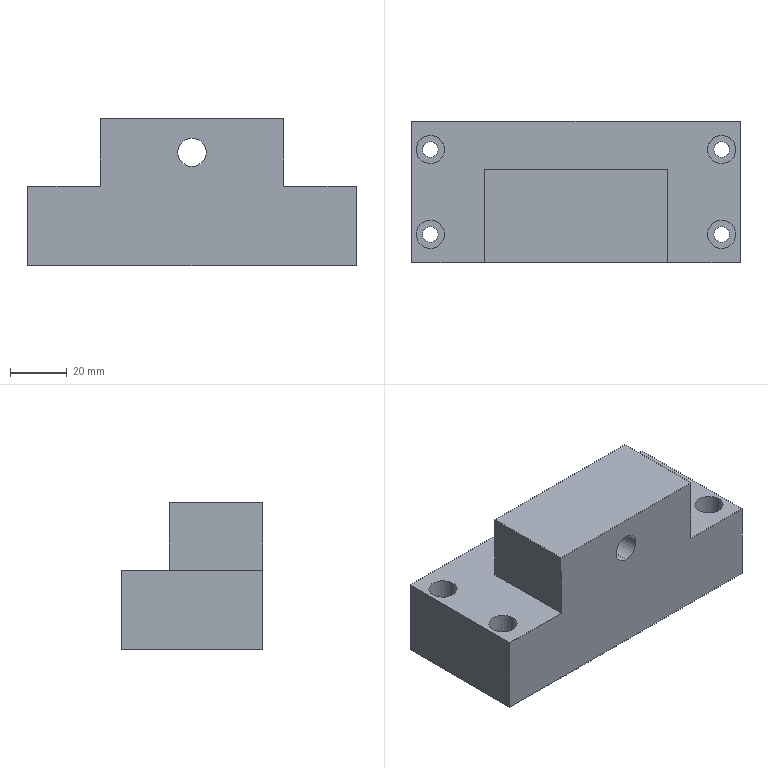Part | 1 solid | 36 faces | box 116 x 50 x 52 mm | volume 203244 mm3 | cylinder 20 | plane 14 | cone 2 | commonest cylinder face diameters 10 x10 5.5 x8 8.5 x2
STEP:
#1=CARTESIAN_POINT('',(46.5,-15.,10.));
#2=VERTEX_POINT('',#1);
#3=CARTESIAN_POINT('',(56.5,-15.,10.));
#4=VERTEX_POINT('',#3);
#5=CARTESIAN_POINT('',(51.5,-15.,10.));
#6=DIRECTION('',(0.,0.,1.));
#7=DIRECTION('',(1.,0.,0.));
#8=AXIS2_PLACEMENT_3D('',#5,#6,#7);
#9=CIRCLE('',#8,5.);
#10=EDGE_CURVE('',#2,#4,#9,.T.);
#11=ORIENTED_EDGE('',*,*,#10,.F.);
#12=CARTESIAN_POINT('',(46.5,-15.,28.));
#13=VERTEX_POINT('',#12);
#14=CARTESIAN_POINT('',(46.5,-15.,28.));
#15=DIRECTION('',(0.,0.,1.));
#16=VECTOR('',#15,1000.);
#17=LINE('',#14,#16);
#18=EDGE_CURVE('',#2,#13,#17,.T.);
#19=ORIENTED_EDGE('',*,*,#18,.T.);
#20=CARTESIAN_POINT('',(56.5,-15.,28.));
#21=VERTEX_POINT('',#20);
#22=CARTESIAN_POINT('',(51.5,-15.,28.));
#23=DIRECTION('',(0.,0.,1.));
#24=DIRECTION('',(1.,0.,0.));
#25=AXIS2_PLACEMENT_3D('',#22,#23,#24);
#26=CIRCLE('',#25,5.);
#27=EDGE_CURVE('',#13,#21,#26,.T.);
#28=ORIENTED_EDGE('',*,*,#27,.T.);
#29=CARTESIAN_POINT('',(56.5,-15.,28.));
#30=DIRECTION('',(0.,0.,1.));
#31=VECTOR('',#30,1000.);
#32=LINE('',#29,#31);
#33=EDGE_CURVE('',#4,#21,#32,.T.);
#34=ORIENTED_EDGE('',*,*,#33,.F.);
#35=EDGE_LOOP('',(#11,#19,#28,#34));
#36=FACE_OUTER_BOUND('',#35,.T.);
#37=CARTESIAN_POINT('',(51.5,-15.,28.));
#38=DIRECTION('',(0.,0.,1.));
#39=DIRECTION('',(1.,0.,0.));
#40=AXIS2_PLACEMENT_3D('',#37,#38,#39);
#41=CYLINDRICAL_SURFACE('',#40,5.);
#42=ADVANCED_FACE('',(#36),#41,.F.);
#43=CARTESIAN_POINT('',(48.75,-15.,0.));
#44=VERTEX_POINT('',#43);
#45=CARTESIAN_POINT('',(54.25,-15.,0.));
#46=VERTEX_POINT('',#45);
#47=CARTESIAN_POINT('',(51.5,-15.,0.));
#48=DIRECTION('',(0.,0.,1.));
#49=DIRECTION('',(1.,0.,0.));
#50=AXIS2_PLACEMENT_3D('',#47,#48,#49);
#51=CIRCLE('',#50,2.75);
#52=EDGE_CURVE('',#44,#46,#51,.T.);
#53=ORIENTED_EDGE('',*,*,#52,.F.);
#54=CARTESIAN_POINT('',(48.75,-15.,10.));
#55=VERTEX_POINT('',#54);
#56=CARTESIAN_POINT('',(48.75,-15.,28.));
#57=DIRECTION('',(0.,0.,1.));
#58=VECTOR('',#57,1000.);
#59=LINE('',#56,#58);
#60=EDGE_CURVE('',#44,#55,#59,.T.);
#61=ORIENTED_EDGE('',*,*,#60,.T.);
#62=CARTESIAN_POINT('',(54.25,-15.,10.));
#63=VERTEX_POINT('',#62);
#64=CARTESIAN_POINT('',(51.5,-15.,10.));
#65=DIRECTION('',(0.,0.,1.));
#66=DIRECTION('',(1.,0.,0.));
#67=AXIS2_PLACEMENT_3D('',#64,#65,#66);
#68=CIRCLE('',#67,2.75);
#69=EDGE_CURVE('',#55,#63,#68,.T.);
#70=ORIENTED_EDGE('',*,*,#69,.T.);
#71=CARTESIAN_POINT('',(54.25,-15.,28.));
#72=DIRECTION('',(0.,0.,1.));
#73=VECTOR('',#72,1000.);
#74=LINE('',#71,#73);
#75=EDGE_CURVE('',#46,#63,#74,.T.);
#76=ORIENTED_EDGE('',*,*,#75,.F.);
#77=EDGE_LOOP('',(#53,#61,#70,#76));
#78=FACE_OUTER_BOUND('',#77,.T.);
#79=CARTESIAN_POINT('',(51.5,-15.,28.));
#80=DIRECTION('',(0.,0.,1.));
#81=DIRECTION('',(1.,0.,0.));
#82=AXIS2_PLACEMENT_3D('',#79,#80,#81);
#83=CYLINDRICAL_SURFACE('',#82,2.75);
#84=ADVANCED_FACE('',(#78),#83,.F.);
#85=CARTESIAN_POINT('',(46.5,15.,10.));
#86=VERTEX_POINT('',#85);
#87=CARTESIAN_POINT('',(56.5,15.,10.));
#88=VERTEX_POINT('',#87);
#89=CARTESIAN_POINT('',(51.5,15.,10.));
#90=DIRECTION('',(0.,0.,1.));
#91=DIRECTION('',(1.,0.,0.));
#92=AXIS2_PLACEMENT_3D('',#89,#90,#91);
#93=CIRCLE('',#92,5.);
#94=EDGE_CURVE('',#86,#88,#93,.T.);
#95=ORIENTED_EDGE('',*,*,#94,.F.);
#96=CARTESIAN_POINT('',(46.5,15.,28.));
#97=VERTEX_POINT('',#96);
#98=CARTESIAN_POINT('',(46.5,15.,28.));
#99=DIRECTION('',(0.,0.,1.));
#100=VECTOR('',#99,1000.);
#101=LINE('',#98,#100);
#102=EDGE_CURVE('',#86,#97,#101,.T.);
#103=ORIENTED_EDGE('',*,*,#102,.T.);
#104=CARTESIAN_POINT('',(56.5,15.,28.));
#105=VERTEX_POINT('',#104);
#106=CARTESIAN_POINT('',(51.5,15.,28.));
#107=DIRECTION('',(0.,0.,1.));
#108=DIRECTION('',(1.,0.,0.));
#109=AXIS2_PLACEMENT_3D('',#106,#107,#108);
#110=CIRCLE('',#109,5.);
#111=EDGE_CURVE('',#97,#105,#110,.T.);
#112=ORIENTED_EDGE('',*,*,#111,.T.);
#113=CARTESIAN_POINT('',(56.5,15.,28.));
#114=DIRECTION('',(0.,0.,1.));
#115=VECTOR('',#114,1000.);
#116=LINE('',#113,#115);
#117=EDGE_CURVE('',#88,#105,#116,.T.);
#118=ORIENTED_EDGE('',*,*,#117,.F.);
#119=EDGE_LOOP('',(#95,#103,#112,#118));
#120=FACE_OUTER_BOUND('',#119,.T.);
#121=CARTESIAN_POINT('',(51.5,15.,28.));
#122=DIRECTION('',(0.,0.,1.));
#123=DIRECTION('',(1.,0.,0.));
#124=AXIS2_PLACEMENT_3D('',#121,#122,#123);
#125=CYLINDRICAL_SURFACE('',#124,5.);
#126=ADVANCED_FACE('',(#120),#125,.F.);
#127=CARTESIAN_POINT('',(48.75,15.,0.));
#128=VERTEX_POINT('',#127);
#129=CARTESIAN_POINT('',(54.25,15.,0.));
#130=VERTEX_POINT('',#129);
#131=CARTESIAN_POINT('',(51.5,15.,0.));
#132=DIRECTION('',(0.,0.,1.));
#133=DIRECTION('',(1.,0.,0.));
#134=AXIS2_PLACEMENT_3D('',#131,#132,#133);
#135=CIRCLE('',#134,2.75);
#136=EDGE_CURVE('',#128,#130,#135,.T.);
#137=ORIENTED_EDGE('',*,*,#136,.F.);
#138=CARTESIAN_POINT('',(48.75,15.,10.));
#139=VERTEX_POINT('',#138);
#140=CARTESIAN_POINT('',(48.75,15.,28.));
#141=DIRECTION('',(0.,0.,1.));
#142=VECTOR('',#141,1000.);
#143=LINE('',#140,#142);
#144=EDGE_CURVE('',#128,#139,#143,.T.);
#145=ORIENTED_EDGE('',*,*,#144,.T.);
#146=CARTESIAN_POINT('',(54.25,15.,10.));
#147=VERTEX_POINT('',#146);
#148=CARTESIAN_POINT('',(51.5,15.,10.));
#149=DIRECTION('',(0.,0.,1.));
#150=DIRECTION('',(1.,0.,0.));
#151=AXIS2_PLACEMENT_3D('',#148,#149,#150);
#152=CIRCLE('',#151,2.75);
#153=EDGE_CURVE('',#139,#147,#152,.T.);
#154=ORIENTED_EDGE('',*,*,#153,.T.);
#155=CARTESIAN_POINT('',(54.25,15.,28.));
#156=DIRECTION('',(0.,0.,1.));
#157=VECTOR('',#156,1000.);
#158=LINE('',#155,#157);
#159=EDGE_CURVE('',#130,#147,#158,.T.);
#160=ORIENTED_EDGE('',*,*,#159,.F.);
#161=EDGE_LOOP('',(#137,#145,#154,#160));
#162=FACE_OUTER_BOUND('',#161,.T.);
#163=CARTESIAN_POINT('',(51.5,15.,28.));
#164=DIRECTION('',(0.,0.,1.));
#165=DIRECTION('',(1.,0.,0.));
#166=AXIS2_PLACEMENT_3D('',#163,#164,#165);
#167=CYLINDRICAL_SURFACE('',#166,2.75);
#168=ADVANCED_FACE('',(#162),#167,.F.);
#169=CARTESIAN_POINT('',(-56.5,-15.,10.));
#170=VERTEX_POINT('',#169);
#171=CARTESIAN_POINT('',(-46.5,-15.,10.));
#172=VERTEX_POINT('',#171);
#173=CARTESIAN_POINT('',(-51.5,-15.,10.));
#174=DIRECTION('',(0.,0.,1.));
#175=DIRECTION('',(1.,0.,0.));
#176=AXIS2_PLACEMENT_3D('',#173,#174,#175);
#177=CIRCLE('',#176,5.);
#178=EDGE_CURVE('',#170,#172,#177,.T.);
#179=ORIENTED_EDGE('',*,*,#178,.F.);
#180=CARTESIAN_POINT('',(-56.5,-15.,28.));
#181=VERTEX_POINT('',#180);
#182=CARTESIAN_POINT('',(-56.5,-15.,28.));
#183=DIRECTION('',(0.,0.,1.));
#184=VECTOR('',#183,1000.);
#185=LINE('',#182,#184);
#186=EDGE_CURVE('',#170,#181,#185,.T.);
#187=ORIENTED_EDGE('',*,*,#186,.T.);
#188=CARTESIAN_POINT('',(-46.5,-15.,28.));
#189=VERTEX_POINT('',#188);
#190=CARTESIAN_POINT('',(-51.5,-15.,28.));
#191=DIRECTION('',(0.,0.,1.));
#192=DIRECTION('',(1.,0.,0.));
#193=AXIS2_PLACEMENT_3D('',#190,#191,#192);
#194=CIRCLE('',#193,5.);
#195=EDGE_CURVE('',#181,#189,#194,.T.);
#196=ORIENTED_EDGE('',*,*,#195,.T.);
#197=CARTESIAN_POINT('',(-46.5,-15.,28.));
#198=DIRECTION('',(0.,0.,1.));
#199=VECTOR('',#198,1000.);
#200=LINE('',#197,#199);
#201=EDGE_CURVE('',#172,#189,#200,.T.);
#202=ORIENTED_EDGE('',*,*,#201,.F.);
#203=EDGE_LOOP('',(#179,#187,#196,#202));
#204=FACE_OUTER_BOUND('',#203,.T.);
#205=CARTESIAN_POINT('',(-51.5,-15.,28.));
#206=DIRECTION('',(0.,0.,1.));
#207=DIRECTION('',(1.,0.,0.));
#208=AXIS2_PLACEMENT_3D('',#205,#206,#207);
#209=CYLINDRICAL_SURFACE('',#208,5.);
#210=ADVANCED_FACE('',(#204),#209,.F.);
#211=CARTESIAN_POINT('',(-54.25,-15.,0.));
#212=VERTEX_POINT('',#211);
#213=CARTESIAN_POINT('',(-48.75,-15.,0.));
#214=VERTEX_POINT('',#213);
#215=CARTESIAN_POINT('',(-51.5,-15.,0.));
#216=DIRECTION('',(0.,0.,1.));
#217=DIRECTION('',(1.,0.,0.));
#218=AXIS2_PLACEMENT_3D('',#215,#216,#217);
#219=CIRCLE('',#218,2.75);
#220=EDGE_CURVE('',#212,#214,#219,.T.);
#221=ORIENTED_EDGE('',*,*,#220,.F.);
#222=CARTESIAN_POINT('',(-54.25,-15.,10.));
#223=VERTEX_POINT('',#222);
#224=CARTESIAN_POINT('',(-54.25,-15.,28.));
#225=DIRECTION('',(0.,0.,1.));
#226=VECTOR('',#225,1000.);
#227=LINE('',#224,#226);
#228=EDGE_CURVE('',#212,#223,#227,.T.);
#229=ORIENTED_EDGE('',*,*,#228,.T.);
#230=CARTESIAN_POINT('',(-48.75,-15.,10.));
#231=VERTEX_POINT('',#230);
#232=CARTESIAN_POINT('',(-51.5,-15.,10.));
#233=DIRECTION('',(0.,0.,1.));
#234=DIRECTION('',(1.,0.,0.));
#235=AXIS2_PLACEMENT_3D('',#232,#233,#234);
#236=CIRCLE('',#235,2.75);
#237=EDGE_CURVE('',#223,#231,#236,.T.);
#238=ORIENTED_EDGE('',*,*,#237,.T.);
#239=CARTESIAN_POINT('',(-48.75,-15.,28.));
#240=DIRECTION('',(0.,0.,1.));
#241=VECTOR('',#240,1000.);
#242=LINE('',#239,#241);
#243=EDGE_CURVE('',#214,#231,#242,.T.);
#244=ORIENTED_EDGE('',*,*,#243,.F.);
#245=EDGE_LOOP('',(#221,#229,#238,#244));
#246=FACE_OUTER_BOUND('',#245,.T.);
#247=CARTESIAN_POINT('',(-51.5,-15.,28.));
#248=DIRECTION('',(0.,0.,1.));
#249=DIRECTION('',(1.,0.,0.));
#250=AXIS2_PLACEMENT_3D('',#247,#248,#249);
#251=CYLINDRICAL_SURFACE('',#250,2.75);
#252=ADVANCED_FACE('',(#246),#251,.F.);
#253=CARTESIAN_POINT('',(-56.5,15.,10.));
#254=VERTEX_POINT('',#253);
#255=CARTESIAN_POINT('',(-46.5,15.,10.));
#256=VERTEX_POINT('',#255);
#257=CARTESIAN_POINT('',(-51.5,15.,10.));
#258=DIRECTION('',(0.,0.,1.));
#259=DIRECTION('',(1.,0.,0.));
#260=AXIS2_PLACEMENT_3D('',#257,#258,#259);
#261=CIRCLE('',#260,5.);
#262=EDGE_CURVE('',#254,#256,#261,.T.);
#263=ORIENTED_EDGE('',*,*,#262,.F.);
#264=CARTESIAN_POINT('',(-56.5,15.,28.));
#265=VERTEX_POINT('',#264);
#266=CARTESIAN_POINT('',(-56.5,15.,28.));
#267=DIRECTION('',(0.,0.,1.));
#268=VECTOR('',#267,1000.);
#269=LINE('',#266,#268);
#270=EDGE_CURVE('',#254,#265,#269,.T.);
#271=ORIENTED_EDGE('',*,*,#270,.T.);
#272=CARTESIAN_POINT('',(-46.5,15.,28.));
#273=VERTEX_POINT('',#272);
#274=CARTESIAN_POINT('',(-51.5,15.,28.));
#275=DIRECTION('',(0.,0.,1.));
#276=DIRECTION('',(1.,0.,0.));
#277=AXIS2_PLACEMENT_3D('',#274,#275,#276);
#278=CIRCLE('',#277,5.);
#279=EDGE_CURVE('',#265,#273,#278,.T.);
#280=ORIENTED_EDGE('',*,*,#279,.T.);
#281=CARTESIAN_POINT('',(-46.5,15.,28.));
#282=DIRECTION('',(0.,0.,1.));
#283=VECTOR('',#282,1000.);
#284=LINE('',#281,#283);
#285=EDGE_CURVE('',#256,#273,#284,.T.);
#286=ORIENTED_EDGE('',*,*,#285,.F.);
#287=EDGE_LOOP('',(#263,#271,#280,#286));
#288=FACE_OUTER_BOUND('',#287,.T.);
#289=CARTESIAN_POINT('',(-51.5,15.,28.));
#290=DIRECTION('',(0.,0.,1.));
#291=DIRECTION('',(1.,0.,0.));
#292=AXIS2_PLACEMENT_3D('',#289,#290,#291);
#293=CYLINDRICAL_SURFACE('',#292,5.);
#294=ADVANCED_FACE('',(#288),#293,.F.);
#295=CARTESIAN_POINT('',(-54.25,15.,0.));
#296=VERTEX_POINT('',#295);
#297=CARTESIAN_POINT('',(-48.75,15.,0.));
#298=VERTEX_POINT('',#297);
#299=CARTESIAN_POINT('',(-51.5,15.,0.));
#300=DIRECTION('',(0.,0.,1.));
#301=DIRECTION('',(1.,0.,0.));
#302=AXIS2_PLACEMENT_3D('',#299,#300,#301);
#303=CIRCLE('',#302,2.75);
#304=EDGE_CURVE('',#296,#298,#303,.T.);
#305=ORIENTED_EDGE('',*,*,#304,.F.);
#306=CARTESIAN_POINT('',(-54.25,15.,10.));
#307=VERTEX_POINT('',#306);
#308=CARTESIAN_POINT('',(-54.25,15.,28.));
#309=DIRECTION('',(0.,0.,1.));
#310=VECTOR('',#309,1000.);
#311=LINE('',#308,#310);
#312=EDGE_CURVE('',#296,#307,#311,.T.);
#313=ORIENTED_EDGE('',*,*,#312,.T.);
#314=CARTESIAN_POINT('',(-48.75,15.,10.));
#315=VERTEX_POINT('',#314);
#316=CARTESIAN_POINT('',(-51.5,15.,10.));
#317=DIRECTION('',(0.,0.,1.));
#318=DIRECTION('',(1.,0.,0.));
#319=AXIS2_PLACEMENT_3D('',#316,#317,#318);
#320=CIRCLE('',#319,2.75);
#321=EDGE_CURVE('',#307,#315,#320,.T.);
#322=ORIENTED_EDGE('',*,*,#321,.T.);
#323=CARTESIAN_POINT('',(-48.75,15.,28.));
#324=DIRECTION('',(0.,0.,1.));
#325=VECTOR('',#324,1000.);
#326=LINE('',#323,#325);
#327=EDGE_CURVE('',#298,#315,#326,.T.);
#328=ORIENTED_EDGE('',*,*,#327,.F.);
#329=EDGE_LOOP('',(#305,#313,#322,#328));
#330=FACE_OUTER_BOUND('',#329,.T.);
#331=CARTESIAN_POINT('',(-51.5,15.,28.));
#332=DIRECTION('',(0.,0.,1.));
#333=DIRECTION('',(1.,0.,0.));
#334=AXIS2_PLACEMENT_3D('',#331,#332,#333);
#335=CYLINDRICAL_SURFACE('',#334,2.75);
#336=ADVANCED_FACE('',(#330),#335,.F.);
#337=CARTESIAN_POINT('',(0.,0.5,5.75));
#338=VERTEX_POINT('',#337);
#339=CARTESIAN_POINT('',(0.,0.5,14.25));
#340=VERTEX_POINT('',#339);
#341=CARTESIAN_POINT('',(0.,0.5,10.));
#342=DIRECTION('',(0.,1.,0.));
#343=DIRECTION('',(0.,0.,1.));
#344=AXIS2_PLACEMENT_3D('',#341,#342,#343);
#345=CIRCLE('',#344,4.25);
#346=EDGE_CURVE('',#338,#340,#345,.T.);
#347=ORIENTED_EDGE('',*,*,#346,.F.);
#348=CARTESIAN_POINT('',(0.,25.,5.75));
#349=VERTEX_POINT('',#348);
#350=CARTESIAN_POINT('',(0.,25.,5.75));
#351=DIRECTION('',(0.,1.,0.));
#352=VECTOR('',#351,1000.);
#353=LINE('',#350,#352);
#354=EDGE_CURVE('',#338,#349,#353,.T.);
#355=ORIENTED_EDGE('',*,*,#354,.T.);
#356=CARTESIAN_POINT('',(0.,25.,14.25));
#357=VERTEX_POINT('',#356);
#358=CARTESIAN_POINT('',(0.,25.,10.));
#359=DIRECTION('',(0.,1.,0.));
#360=DIRECTION('',(0.,0.,1.));
#361=AXIS2_PLACEMENT_3D('',#358,#359,#360);
#362=CIRCLE('',#361,4.25);
#363=EDGE_CURVE('',#349,#357,#362,.T.);
#364=ORIENTED_EDGE('',*,*,#363,.T.);
#365=CARTESIAN_POINT('',(0.,25.,14.25));
#366=DIRECTION('',(0.,1.,0.));
#367=VECTOR('',#366,1000.);
#368=LINE('',#365,#367);
#369=EDGE_CURVE('',#340,#357,#368,.T.);
#370=ORIENTED_EDGE('',*,*,#369,.F.);
#371=EDGE_LOOP('',(#347,#355,#364,#370));
#372=FACE_OUTER_BOUND('',#371,.T.);
#373=CARTESIAN_POINT('',(0.,25.,10.));
#374=DIRECTION('',(0.,1.,0.));
#375=DIRECTION('',(0.,0.,1.));
#376=AXIS2_PLACEMENT_3D('',#373,#374,#375);
#377=CYLINDRICAL_SURFACE('',#376,4.25);
#378=ADVANCED_FACE('',(#372),#377,.F.);
#379=CARTESIAN_POINT('',(0.,-2.054,10.));
#380=VERTEX_POINT('',#379);
#381=CARTESIAN_POINT('',(0.,0.5,14.25));
#382=DIRECTION('',(0.,0.515,0.8572));
#383=VECTOR('',#382,1000.);
#384=LINE('',#381,#383);
#385=EDGE_CURVE('',#380,#340,#384,.T.);
#386=ORIENTED_EDGE('',*,*,#385,.F.);
#387=CARTESIAN_POINT('',(0.,0.5,5.75));
#388=DIRECTION('',(0.,0.515,-0.8572));
#389=VECTOR('',#388,1000.);
#390=LINE('',#387,#389);
#391=EDGE_CURVE('',#380,#338,#390,.T.);
#392=ORIENTED_EDGE('',*,*,#391,.T.);
#393=ORIENTED_EDGE('',*,*,#346,.T.);
#394=EDGE_LOOP('',(#386,#392,#393));
#395=FACE_OUTER_BOUND('',#394,.T.);
#396=CARTESIAN_POINT('',(0.,0.5,10.));
#397=DIRECTION('',(0.,1.,0.));
#398=DIRECTION('',(0.,0.,1.));
#399=AXIS2_PLACEMENT_3D('',#396,#397,#398);
#400=CONICAL_SURFACE('',#399,4.25,1.03);
#401=ADVANCED_FACE('',(#395),#400,.F.);
#402=CARTESIAN_POINT('',(0.,-25.,35.));
#403=VERTEX_POINT('',#402);
#404=CARTESIAN_POINT('',(0.,-25.,45.));
#405=VERTEX_POINT('',#404);
#406=CARTESIAN_POINT('',(0.,-25.,40.));
#407=DIRECTION('',(0.,1.,0.));
#408=DIRECTION('',(0.,0.,1.));
#409=AXIS2_PLACEMENT_3D('',#406,#407,#408);
#410=CIRCLE('',#409,5.);
#411=EDGE_CURVE('',#403,#405,#410,.T.);
#412=ORIENTED_EDGE('',*,*,#411,.F.);
#413=CARTESIAN_POINT('',(0.,8.,35.));
#414=VERTEX_POINT('',#413);
#415=CARTESIAN_POINT('',(0.,8.,35.));
#416=DIRECTION('',(0.,1.,0.));
#417=VECTOR('',#416,1000.);
#418=LINE('',#415,#417);
#419=EDGE_CURVE('',#403,#414,#418,.T.);
#420=ORIENTED_EDGE('',*,*,#419,.T.);
#421=CARTESIAN_POINT('',(0.,8.,45.));
#422=VERTEX_POINT('',#421);
#423=CARTESIAN_POINT('',(0.,8.,40.));
#424=DIRECTION('',(0.,1.,0.));
#425=DIRECTION('',(0.,0.,1.));
#426=AXIS2_PLACEMENT_3D('',#423,#424,#425);
#427=CIRCLE('',#426,5.);
#428=EDGE_CURVE('',#414,#422,#427,.T.);
#429=ORIENTED_EDGE('',*,*,#428,.T.);
#430=CARTESIAN_POINT('',(0.,8.,45.));
#431=DIRECTION('',(0.,1.,0.));
#432=VECTOR('',#431,1000.);
#433=LINE('',#430,#432);
#434=EDGE_CURVE('',#405,#422,#433,.T.);
#435=ORIENTED_EDGE('',*,*,#434,.F.);
#436=EDGE_LOOP('',(#412,#420,#429,#435));
#437=FACE_OUTER_BOUND('',#436,.T.);
#438=CARTESIAN_POINT('',(0.,8.,40.));
#439=DIRECTION('',(0.,1.,0.));
#440=DIRECTION('',(0.,0.,1.));
#441=AXIS2_PLACEMENT_3D('',#438,#439,#440);
#442=CYLINDRICAL_SURFACE('',#441,5.);
#443=ADVANCED_FACE('',(#437),#442,.F.);
#444=CARTESIAN_POINT('',(51.5,-15.,28.));
#445=DIRECTION('',(0.,0.,1.));
#446=DIRECTION('',(1.,0.,0.));
#447=AXIS2_PLACEMENT_3D('',#444,#445,#446);
#448=CIRCLE('',#447,5.);
#449=EDGE_CURVE('',#21,#13,#448,.T.);
#450=ORIENTED_EDGE('',*,*,#449,.F.);
#451=ORIENTED_EDGE('',*,*,#27,.F.);
#452=EDGE_LOOP('',(#450,#451));
#453=FACE_BOUND('',#452,.T.);
#454=CARTESIAN_POINT('',(51.5,15.,28.));
#455=DIRECTION('',(0.,0.,1.));
#456=DIRECTION('',(1.,0.,0.));
#457=AXIS2_PLACEMENT_3D('',#454,#455,#456);
#458=CIRCLE('',#457,5.);
#459=EDGE_CURVE('',#105,#97,#458,.T.);
#460=ORIENTED_EDGE('',*,*,#459,.F.);
#461=ORIENTED_EDGE('',*,*,#111,.F.);
#462=EDGE_LOOP('',(#460,#461));
#463=FACE_BOUND('',#462,.T.);
#464=CARTESIAN_POINT('',(-51.5,-15.,28.));
#465=DIRECTION('',(0.,0.,1.));
#466=DIRECTION('',(1.,0.,0.));
#467=AXIS2_PLACEMENT_3D('',#464,#465,#466);
#468=CIRCLE('',#467,5.);
#469=EDGE_CURVE('',#189,#181,#468,.T.);
#470=ORIENTED_EDGE('',*,*,#469,.F.);
#471=ORIENTED_EDGE('',*,*,#195,.F.);
#472=EDGE_LOOP('',(#470,#471));
#473=FACE_BOUND('',#472,.T.);
#474=CARTESIAN_POINT('',(-51.5,15.,28.));
#475=DIRECTION('',(0.,0.,1.));
#476=DIRECTION('',(1.,0.,0.));
#477=AXIS2_PLACEMENT_3D('',#474,#475,#476);
#478=CIRCLE('',#477,5.);
#479=EDGE_CURVE('',#273,#265,#478,.T.);
#480=ORIENTED_EDGE('',*,*,#479,.F.);
#481=ORIENTED_EDGE('',*,*,#279,.F.);
#482=EDGE_LOOP('',(#480,#481));
#483=FACE_BOUND('',#482,.T.);
#484=CARTESIAN_POINT('',(-32.5,8.,28.));
#485=VERTEX_POINT('',#484);
#486=CARTESIAN_POINT('',(-32.5,-25.,28.));
#487=VERTEX_POINT('',#486);
#488=CARTESIAN_POINT('',(-32.5,-25.,28.));
#489=DIRECTION('',(0.,-1.,0.));
#490=VECTOR('',#489,1000.);
#491=LINE('',#488,#490);
#492=EDGE_CURVE('',#485,#487,#491,.T.);
#493=ORIENTED_EDGE('',*,*,#492,.F.);
#494=CARTESIAN_POINT('',(32.5,8.,28.));
#495=VERTEX_POINT('',#494);
#496=CARTESIAN_POINT('',(-32.5,8.,28.));
#497=DIRECTION('',(-1.,0.,0.));
#498=VECTOR('',#497,1000.);
#499=LINE('',#496,#498);
#500=EDGE_CURVE('',#495,#485,#499,.T.);
#501=ORIENTED_EDGE('',*,*,#500,.F.);
#502=CARTESIAN_POINT('',(32.5,-25.,28.));
#503=VERTEX_POINT('',#502);
#504=CARTESIAN_POINT('',(32.5,8.,28.));
#505=DIRECTION('',(0.,1.,0.));
#506=VECTOR('',#505,1000.);
#507=LINE('',#504,#506);
#508=EDGE_CURVE('',#503,#495,#507,.T.);
#509=ORIENTED_EDGE('',*,*,#508,.F.);
#510=CARTESIAN_POINT('',(58.,-25.,28.));
#511=VERTEX_POINT('',#510);
#512=CARTESIAN_POINT('',(58.,-25.,28.));
#513=DIRECTION('',(-1.,0.,0.));
#514=VECTOR('',#513,1000.);
#515=LINE('',#512,#514);
#516=EDGE_CURVE('',#511,#503,#515,.T.);
#517=ORIENTED_EDGE('',*,*,#516,.F.);
#518=CARTESIAN_POINT('',(58.,25.,28.));
#519=VERTEX_POINT('',#518);
#520=CARTESIAN_POINT('',(58.,25.,28.));
#521=DIRECTION('',(0.,-1.,0.));
#522=VECTOR('',#521,1000.);
#523=LINE('',#520,#522);
#524=EDGE_CURVE('',#519,#511,#523,.T.);
#525=ORIENTED_EDGE('',*,*,#524,.F.);
#526=CARTESIAN_POINT('',(-58.,25.,28.));
#527=VERTEX_POINT('',#526);
#528=CARTESIAN_POINT('',(-58.,25.,28.));
#529=DIRECTION('',(1.,0.,0.));
#530=VECTOR('',#529,1000.);
#531=LINE('',#528,#530);
#532=EDGE_CURVE('',#527,#519,#531,.T.);
#533=ORIENTED_EDGE('',*,*,#532,.F.);
#534=CARTESIAN_POINT('',(-58.,-25.,28.));
#535=VERTEX_POINT('',#534);
#536=CARTESIAN_POINT('',(-58.,-25.,28.));
#537=DIRECTION('',(0.,1.,0.));
#538=VECTOR('',#537,1000.);
#539=LINE('',#536,#538);
#540=EDGE_CURVE('',#535,#527,#539,.T.);
#541=ORIENTED_EDGE('',*,*,#540,.F.);
#542=CARTESIAN_POINT('',(58.,-25.,28.));
#543=DIRECTION('',(-1.,0.,0.));
#544=VECTOR('',#543,1000.);
#545=LINE('',#542,#544);
#546=EDGE_CURVE('',#487,#535,#545,.T.);
#547=ORIENTED_EDGE('',*,*,#546,.F.);
#548=EDGE_LOOP('',(#493,#501,#509,#517,#525,#533,#541,#547));
#549=FACE_OUTER_BOUND('',#548,.T.);
#550=CARTESIAN_POINT('',(0.,0.,28.));
#551=DIRECTION('',(0.,0.,-1.));
#552=DIRECTION('',(-1.,0.,0.));
#553=AXIS2_PLACEMENT_3D('',#550,#551,#552);
#554=PLANE('',#553);
#555=ADVANCED_FACE('',(#453,#463,#473,#483,#549),#554,.F.);
#556=CARTESIAN_POINT('',(0.,25.,10.));
#557=DIRECTION('',(0.,1.,0.));
#558=DIRECTION('',(0.,0.,1.));
#559=AXIS2_PLACEMENT_3D('',#556,#557,#558);
#560=CIRCLE('',#559,4.25);
#561=EDGE_CURVE('',#357,#349,#560,.T.);
#562=ORIENTED_EDGE('',*,*,#561,.F.);
#563=ORIENTED_EDGE('',*,*,#363,.F.);
#564=EDGE_LOOP('',(#562,#563));
#565=FACE_BOUND('',#564,.T.);
#566=CARTESIAN_POINT('',(-58.,25.,0.));
#567=VERTEX_POINT('',#566);
#568=CARTESIAN_POINT('',(58.,25.,0.));
#569=VERTEX_POINT('',#568);
#570=CARTESIAN_POINT('',(-58.,25.,0.));
#571=DIRECTION('',(1.,0.,0.));
#572=VECTOR('',#571,1000.);
#573=LINE('',#570,#572);
#574=EDGE_CURVE('',#567,#569,#573,.T.);
#575=ORIENTED_EDGE('',*,*,#574,.F.);
#576=CARTESIAN_POINT('',(-58.,25.,28.));
#577=DIRECTION('',(0.,0.,-1.));
#578=VECTOR('',#577,1000.);
#579=LINE('',#576,#578);
#580=EDGE_CURVE('',#527,#567,#579,.T.);
#581=ORIENTED_EDGE('',*,*,#580,.F.);
#582=ORIENTED_EDGE('',*,*,#532,.T.);
#583=CARTESIAN_POINT('',(58.,25.,28.));
#584=DIRECTION('',(0.,0.,-1.));
#585=VECTOR('',#584,1000.);
#586=LINE('',#583,#585);
#587=EDGE_CURVE('',#519,#569,#586,.T.);
#588=ORIENTED_EDGE('',*,*,#587,.T.);
#589=EDGE_LOOP('',(#575,#581,#582,#588));
#590=FACE_OUTER_BOUND('',#589,.T.);
#591=CARTESIAN_POINT('',(-58.,25.,28.));
#592=DIRECTION('',(0.,1.,0.));
#593=DIRECTION('',(0.,0.,1.));
#594=AXIS2_PLACEMENT_3D('',#591,#592,#593);
#595=PLANE('',#594);
#596=ADVANCED_FACE('',(#565,#590),#595,.T.);
#597=CARTESIAN_POINT('',(-58.,-25.,0.));
#598=VERTEX_POINT('',#597);
#599=CARTESIAN_POINT('',(-58.,-25.,0.));
#600=DIRECTION('',(0.,1.,0.));
#601=VECTOR('',#600,1000.);
#602=LINE('',#599,#601);
#603=EDGE_CURVE('',#598,#567,#602,.T.);
#604=ORIENTED_EDGE('',*,*,#603,.F.);
#605=CARTESIAN_POINT('',(-58.,-25.,28.));
#606=DIRECTION('',(0.,0.,-1.));
#607=VECTOR('',#606,1000.);
#608=LINE('',#605,#607);
#609=EDGE_CURVE('',#535,#598,#608,.T.);
#610=ORIENTED_EDGE('',*,*,#609,.F.);
#611=ORIENTED_EDGE('',*,*,#540,.T.);
#612=ORIENTED_EDGE('',*,*,#580,.T.);
#613=EDGE_LOOP('',(#604,#610,#611,#612));
#614=FACE_OUTER_BOUND('',#613,.T.);
#615=CARTESIAN_POINT('',(-58.,-25.,28.));
#616=DIRECTION('',(-1.,0.,0.));
#617=DIRECTION('',(0.,0.,1.));
#618=AXIS2_PLACEMENT_3D('',#615,#616,#617);
#619=PLANE('',#618);
#620=ADVANCED_FACE('',(#614),#619,.T.);
#621=CARTESIAN_POINT('',(0.,-25.,40.));
#622=DIRECTION('',(0.,1.,0.));
#623=DIRECTION('',(0.,0.,1.));
#624=AXIS2_PLACEMENT_3D('',#621,#622,#623);
#625=CIRCLE('',#624,5.);
#626=EDGE_CURVE('',#405,#403,#625,.T.);
#627=ORIENTED_EDGE('',*,*,#626,.T.);
#628=ORIENTED_EDGE('',*,*,#411,.T.);
#629=EDGE_LOOP('',(#627,#628));
#630=FACE_BOUND('',#629,.T.);
#631=CARTESIAN_POINT('',(58.,-25.,0.));
#632=VERTEX_POINT('',#631);
#633=CARTESIAN_POINT('',(58.,-25.,0.));
#634=DIRECTION('',(-1.,0.,0.));
#635=VECTOR('',#634,1000.);
#636=LINE('',#633,#635);
#637=EDGE_CURVE('',#632,#598,#636,.T.);
#638=ORIENTED_EDGE('',*,*,#637,.F.);
#639=CARTESIAN_POINT('',(58.,-25.,28.));
#640=DIRECTION('',(0.,0.,-1.));
#641=VECTOR('',#640,1000.);
#642=LINE('',#639,#641);
#643=EDGE_CURVE('',#511,#632,#642,.T.);
#644=ORIENTED_EDGE('',*,*,#643,.F.);
#645=ORIENTED_EDGE('',*,*,#516,.T.);
#646=CARTESIAN_POINT('',(32.5,-25.,52.));
#647=VERTEX_POINT('',#646);
#648=CARTESIAN_POINT('',(32.5,-25.,52.));
#649=DIRECTION('',(0.,0.,-1.));
#650=VECTOR('',#649,1000.);
#651=LINE('',#648,#650);
#652=EDGE_CURVE('',#647,#503,#651,.T.);
#653=ORIENTED_EDGE('',*,*,#652,.F.);
#654=CARTESIAN_POINT('',(-32.5,-25.,52.));
#655=VERTEX_POINT('',#654);
#656=CARTESIAN_POINT('',(32.5,-25.,52.));
#657=DIRECTION('',(1.,0.,0.));
#658=VECTOR('',#657,1000.);
#659=LINE('',#656,#658);
#660=EDGE_CURVE('',#655,#647,#659,.T.);
#661=ORIENTED_EDGE('',*,*,#660,.F.);
#662=CARTESIAN_POINT('',(-32.5,-25.,52.));
#663=DIRECTION('',(0.,0.,-1.));
#664=VECTOR('',#663,1000.);
#665=LINE('',#662,#664);
#666=EDGE_CURVE('',#655,#487,#665,.T.);
#667=ORIENTED_EDGE('',*,*,#666,.T.);
#668=ORIENTED_EDGE('',*,*,#546,.T.);
#669=ORIENTED_EDGE('',*,*,#609,.T.);
#670=EDGE_LOOP('',(#638,#644,#645,#653,#661,#667,#668,#669));
#671=FACE_OUTER_BOUND('',#670,.T.);
#672=CARTESIAN_POINT('',(58.,-25.,28.));
#673=DIRECTION('',(0.,-1.,0.));
#674=DIRECTION('',(0.,0.,-1.));
#675=AXIS2_PLACEMENT_3D('',#672,#673,#674);
#676=PLANE('',#675);
#677=ADVANCED_FACE('',(#630,#671),#676,.T.);
#678=CARTESIAN_POINT('',(58.,25.,0.));
#679=DIRECTION('',(0.,-1.,0.));
#680=VECTOR('',#679,1000.);
#681=LINE('',#678,#680);
#682=EDGE_CURVE('',#569,#632,#681,.T.);
#683=ORIENTED_EDGE('',*,*,#682,.F.);
#684=ORIENTED_EDGE('',*,*,#587,.F.);
#685=ORIENTED_EDGE('',*,*,#524,.T.);
#686=ORIENTED_EDGE('',*,*,#643,.T.);
#687=EDGE_LOOP('',(#683,#684,#685,#686));
#688=FACE_OUTER_BOUND('',#687,.T.);
#689=CARTESIAN_POINT('',(58.,25.,28.));
#690=DIRECTION('',(1.,0.,0.));
#691=DIRECTION('',(0.,0.,-1.));
#692=AXIS2_PLACEMENT_3D('',#689,#690,#691);
#693=PLANE('',#692);
#694=ADVANCED_FACE('',(#688),#693,.T.);
#695=CARTESIAN_POINT('',(51.5,-15.,0.));
#696=DIRECTION('',(0.,0.,1.));
#697=DIRECTION('',(1.,0.,0.));
#698=AXIS2_PLACEMENT_3D('',#695,#696,#697);
#699=CIRCLE('',#698,2.75);
#700=EDGE_CURVE('',#46,#44,#699,.T.);
#701=ORIENTED_EDGE('',*,*,#700,.T.);
#702=ORIENTED_EDGE('',*,*,#52,.T.);
#703=EDGE_LOOP('',(#701,#702));
#704=FACE_BOUND('',#703,.T.);
#705=CARTESIAN_POINT('',(51.5,15.,0.));
#706=DIRECTION('',(0.,0.,1.));
#707=DIRECTION('',(1.,0.,0.));
#708=AXIS2_PLACEMENT_3D('',#705,#706,#707);
#709=CIRCLE('',#708,2.75);
#710=EDGE_CURVE('',#130,#128,#709,.T.);
#711=ORIENTED_EDGE('',*,*,#710,.T.);
#712=ORIENTED_EDGE('',*,*,#136,.T.);
#713=EDGE_LOOP('',(#711,#712));
#714=FACE_BOUND('',#713,.T.);
#715=CARTESIAN_POINT('',(-51.5,-15.,0.));
#716=DIRECTION('',(0.,0.,1.));
#717=DIRECTION('',(1.,0.,0.));
#718=AXIS2_PLACEMENT_3D('',#715,#716,#717);
#719=CIRCLE('',#718,2.75);
#720=EDGE_CURVE('',#214,#212,#719,.T.);
#721=ORIENTED_EDGE('',*,*,#720,.T.);
#722=ORIENTED_EDGE('',*,*,#220,.T.);
#723=EDGE_LOOP('',(#721,#722));
#724=FACE_BOUND('',#723,.T.);
#725=CARTESIAN_POINT('',(-51.5,15.,0.));
#726=DIRECTION('',(0.,0.,1.));
#727=DIRECTION('',(1.,0.,0.));
#728=AXIS2_PLACEMENT_3D('',#725,#726,#727);
#729=CIRCLE('',#728,2.75);
#730=EDGE_CURVE('',#298,#296,#729,.T.);
#731=ORIENTED_EDGE('',*,*,#730,.T.);
#732=ORIENTED_EDGE('',*,*,#304,.T.);
#733=EDGE_LOOP('',(#731,#732));
#734=FACE_BOUND('',#733,.T.);
#735=ORIENTED_EDGE('',*,*,#574,.T.);
#736=ORIENTED_EDGE('',*,*,#682,.T.);
#737=ORIENTED_EDGE('',*,*,#637,.T.);
#738=ORIENTED_EDGE('',*,*,#603,.T.);
#739=EDGE_LOOP('',(#735,#736,#737,#738));
#740=FACE_OUTER_BOUND('',#739,.T.);
#741=CARTESIAN_POINT('',(0.,0.,0.));
#742=DIRECTION('',(0.,0.,-1.));
#743=DIRECTION('',(-1.,0.,0.));
#744=AXIS2_PLACEMENT_3D('',#741,#742,#743);
#745=PLANE('',#744);
#746=ADVANCED_FACE('',(#704,#714,#724,#734,#740),#745,.T.);
#747=ORIENTED_EDGE('',*,*,#508,.T.);
#748=CARTESIAN_POINT('',(32.5,8.,52.));
#749=VERTEX_POINT('',#748);
#750=CARTESIAN_POINT('',(32.5,8.,52.));
#751=DIRECTION('',(0.,0.,-1.));
#752=VECTOR('',#751,1000.);
#753=LINE('',#750,#752);
#754=EDGE_CURVE('',#749,#495,#753,.T.);
#755=ORIENTED_EDGE('',*,*,#754,.F.);
#756=CARTESIAN_POINT('',(32.5,8.,52.));
#757=DIRECTION('',(0.,1.,0.));
#758=VECTOR('',#757,1000.);
#759=LINE('',#756,#758);
#760=EDGE_CURVE('',#647,#749,#759,.T.);
#761=ORIENTED_EDGE('',*,*,#760,.F.);
#762=ORIENTED_EDGE('',*,*,#652,.T.);
#763=EDGE_LOOP('',(#747,#755,#761,#762));
#764=FACE_OUTER_BOUND('',#763,.T.);
#765=CARTESIAN_POINT('',(32.5,8.,52.));
#766=DIRECTION('',(-1.,0.,0.));
#767=DIRECTION('',(0.,0.,1.));
#768=AXIS2_PLACEMENT_3D('',#765,#766,#767);
#769=PLANE('',#768);
#770=ADVANCED_FACE('',(#764),#769,.F.);
#771=CARTESIAN_POINT('',(0.,8.,40.));
#772=DIRECTION('',(0.,1.,0.));
#773=DIRECTION('',(0.,0.,1.));
#774=AXIS2_PLACEMENT_3D('',#771,#772,#773);
#775=CIRCLE('',#774,5.);
#776=EDGE_CURVE('',#422,#414,#775,.T.);
#777=ORIENTED_EDGE('',*,*,#776,.F.);
#778=ORIENTED_EDGE('',*,*,#428,.F.);
#779=EDGE_LOOP('',(#777,#778));
#780=FACE_BOUND('',#779,.T.);
#781=ORIENTED_EDGE('',*,*,#500,.T.);
#782=CARTESIAN_POINT('',(-32.5,8.,52.));
#783=VERTEX_POINT('',#782);
#784=CARTESIAN_POINT('',(-32.5,8.,52.));
#785=DIRECTION('',(0.,0.,-1.));
#786=VECTOR('',#785,1000.);
#787=LINE('',#784,#786);
#788=EDGE_CURVE('',#783,#485,#787,.T.);
#789=ORIENTED_EDGE('',*,*,#788,.F.);
#790=CARTESIAN_POINT('',(-32.5,8.,52.));
#791=DIRECTION('',(-1.,0.,0.));
#792=VECTOR('',#791,1000.);
#793=LINE('',#790,#792);
#794=EDGE_CURVE('',#749,#783,#793,.T.);
#795=ORIENTED_EDGE('',*,*,#794,.F.);
#796=ORIENTED_EDGE('',*,*,#754,.T.);
#797=EDGE_LOOP('',(#781,#789,#795,#796));
#798=FACE_OUTER_BOUND('',#797,.T.);
#799=CARTESIAN_POINT('',(-32.5,8.,52.));
#800=DIRECTION('',(0.,-1.,0.));
#801=DIRECTION('',(0.,0.,-1.));
#802=AXIS2_PLACEMENT_3D('',#799,#800,#801);
#803=PLANE('',#802);
#804=ADVANCED_FACE('',(#780,#798),#803,.F.);
#805=ORIENTED_EDGE('',*,*,#492,.T.);
#806=ORIENTED_EDGE('',*,*,#666,.F.);
#807=CARTESIAN_POINT('',(-32.5,-25.,52.));
#808=DIRECTION('',(0.,-1.,0.));
#809=VECTOR('',#808,1000.);
#810=LINE('',#807,#809);
#811=EDGE_CURVE('',#783,#655,#810,.T.);
#812=ORIENTED_EDGE('',*,*,#811,.F.);
#813=ORIENTED_EDGE('',*,*,#788,.T.);
#814=EDGE_LOOP('',(#805,#806,#812,#813));
#815=FACE_OUTER_BOUND('',#814,.T.);
#816=CARTESIAN_POINT('',(-32.5,-25.,52.));
#817=DIRECTION('',(1.,0.,0.));
#818=DIRECTION('',(0.,0.,-1.));
#819=AXIS2_PLACEMENT_3D('',#816,#817,#818);
#820=PLANE('',#819);
#821=ADVANCED_FACE('',(#815),#820,.F.);
#822=ORIENTED_EDGE('',*,*,#660,.T.);
#823=ORIENTED_EDGE('',*,*,#760,.T.);
#824=ORIENTED_EDGE('',*,*,#794,.T.);
#825=ORIENTED_EDGE('',*,*,#811,.T.);
#826=EDGE_LOOP('',(#822,#823,#824,#825));
#827=FACE_OUTER_BOUND('',#826,.T.);
#828=CARTESIAN_POINT('',(0.,0.,52.));
#829=DIRECTION('',(0.,0.,-1.));
#830=DIRECTION('',(-1.,0.,0.));
#831=AXIS2_PLACEMENT_3D('',#828,#829,#830);
#832=PLANE('',#831);
#833=ADVANCED_FACE('',(#827),#832,.F.);
#834=ORIENTED_EDGE('',*,*,#419,.F.);
#835=ORIENTED_EDGE('',*,*,#626,.F.);
#836=ORIENTED_EDGE('',*,*,#434,.T.);
#837=ORIENTED_EDGE('',*,*,#776,.T.);
#838=EDGE_LOOP('',(#834,#835,#836,#837));
#839=FACE_OUTER_BOUND('',#838,.T.);
#840=CARTESIAN_POINT('',(0.,8.,40.));
#841=DIRECTION('',(0.,1.,0.));
#842=DIRECTION('',(0.,0.,1.));
#843=AXIS2_PLACEMENT_3D('',#840,#841,#842);
#844=CYLINDRICAL_SURFACE('',#843,5.);
#845=ADVANCED_FACE('',(#839),#844,.F.);
#846=ORIENTED_EDGE('',*,*,#391,.F.);
#847=ORIENTED_EDGE('',*,*,#385,.T.);
#848=CARTESIAN_POINT('',(0.,0.5,10.));
#849=DIRECTION('',(0.,1.,0.));
#850=DIRECTION('',(0.,0.,1.));
#851=AXIS2_PLACEMENT_3D('',#848,#849,#850);
#852=CIRCLE('',#851,4.25);
#853=EDGE_CURVE('',#340,#338,#852,.T.);
#854=ORIENTED_EDGE('',*,*,#853,.T.);
#855=EDGE_LOOP('',(#846,#847,#854));
#856=FACE_OUTER_BOUND('',#855,.T.);
#857=CARTESIAN_POINT('',(0.,0.5,10.));
#858=DIRECTION('',(0.,1.,0.));
#859=DIRECTION('',(0.,0.,1.));
#860=AXIS2_PLACEMENT_3D('',#857,#858,#859);
#861=CONICAL_SURFACE('',#860,4.25,1.03);
#862=ADVANCED_FACE('',(#856),#861,.F.);
#863=ORIENTED_EDGE('',*,*,#354,.F.);
#864=ORIENTED_EDGE('',*,*,#853,.F.);
#865=ORIENTED_EDGE('',*,*,#369,.T.);
#866=ORIENTED_EDGE('',*,*,#561,.T.);
#867=EDGE_LOOP('',(#863,#864,#865,#866));
#868=FACE_OUTER_BOUND('',#867,.T.);
#869=CARTESIAN_POINT('',(0.,25.,10.));
#870=DIRECTION('',(0.,1.,0.));
#871=DIRECTION('',(0.,0.,1.));
#872=AXIS2_PLACEMENT_3D('',#869,#870,#871);
#873=CYLINDRICAL_SURFACE('',#872,4.25);
#874=ADVANCED_FACE('',(#868),#873,.F.);
#875=ORIENTED_EDGE('',*,*,#312,.F.);
#876=ORIENTED_EDGE('',*,*,#730,.F.);
#877=ORIENTED_EDGE('',*,*,#327,.T.);
#878=CARTESIAN_POINT('',(-51.5,15.,10.));
#879=DIRECTION('',(0.,0.,1.));
#880=DIRECTION('',(1.,0.,0.));
#881=AXIS2_PLACEMENT_3D('',#878,#879,#880);
#882=CIRCLE('',#881,2.75);
#883=EDGE_CURVE('',#315,#307,#882,.T.);
#884=ORIENTED_EDGE('',*,*,#883,.T.);
#885=EDGE_LOOP('',(#875,#876,#877,#884));
#886=FACE_OUTER_BOUND('',#885,.T.);
#887=CARTESIAN_POINT('',(-51.5,15.,28.));
#888=DIRECTION('',(0.,0.,1.));
#889=DIRECTION('',(1.,0.,0.));
#890=AXIS2_PLACEMENT_3D('',#887,#888,#889);
#891=CYLINDRICAL_SURFACE('',#890,2.75);
#892=ADVANCED_FACE('',(#886),#891,.F.);
#893=ORIENTED_EDGE('',*,*,#883,.F.);
#894=ORIENTED_EDGE('',*,*,#321,.F.);
#895=EDGE_LOOP('',(#893,#894));
#896=FACE_BOUND('',#895,.T.);
#897=CARTESIAN_POINT('',(-51.5,15.,10.));
#898=DIRECTION('',(0.,0.,1.));
#899=DIRECTION('',(1.,0.,0.));
#900=AXIS2_PLACEMENT_3D('',#897,#898,#899);
#901=CIRCLE('',#900,5.);
#902=EDGE_CURVE('',#256,#254,#901,.T.);
#903=ORIENTED_EDGE('',*,*,#902,.T.);
#904=ORIENTED_EDGE('',*,*,#262,.T.);
#905=EDGE_LOOP('',(#903,#904));
#906=FACE_OUTER_BOUND('',#905,.T.);
#907=CARTESIAN_POINT('',(-48.75,15.,10.));
#908=DIRECTION('',(0.,0.,-1.));
#909=DIRECTION('',(-1.,0.,0.));
#910=AXIS2_PLACEMENT_3D('',#907,#908,#909);
#911=PLANE('',#910);
#912=ADVANCED_FACE('',(#896,#906),#911,.F.);
#913=ORIENTED_EDGE('',*,*,#270,.F.);
#914=ORIENTED_EDGE('',*,*,#902,.F.);
#915=ORIENTED_EDGE('',*,*,#285,.T.);
#916=ORIENTED_EDGE('',*,*,#479,.T.);
#917=EDGE_LOOP('',(#913,#914,#915,#916));
#918=FACE_OUTER_BOUND('',#917,.T.);
#919=CARTESIAN_POINT('',(-51.5,15.,28.));
#920=DIRECTION('',(0.,0.,1.));
#921=DIRECTION('',(1.,0.,0.));
#922=AXIS2_PLACEMENT_3D('',#919,#920,#921);
#923=CYLINDRICAL_SURFACE('',#922,5.);
#924=ADVANCED_FACE('',(#918),#923,.F.);
#925=ORIENTED_EDGE('',*,*,#228,.F.);
#926=ORIENTED_EDGE('',*,*,#720,.F.);
#927=ORIENTED_EDGE('',*,*,#243,.T.);
#928=CARTESIAN_POINT('',(-51.5,-15.,10.));
#929=DIRECTION('',(0.,0.,1.));
#930=DIRECTION('',(1.,0.,0.));
#931=AXIS2_PLACEMENT_3D('',#928,#929,#930);
#932=CIRCLE('',#931,2.75);
#933=EDGE_CURVE('',#231,#223,#932,.T.);
#934=ORIENTED_EDGE('',*,*,#933,.T.);
#935=EDGE_LOOP('',(#925,#926,#927,#934));
#936=FACE_OUTER_BOUND('',#935,.T.);
#937=CARTESIAN_POINT('',(-51.5,-15.,28.));
#938=DIRECTION('',(0.,0.,1.));
#939=DIRECTION('',(1.,0.,0.));
#940=AXIS2_PLACEMENT_3D('',#937,#938,#939);
#941=CYLINDRICAL_SURFACE('',#940,2.75);
#942=ADVANCED_FACE('',(#936),#941,.F.);
#943=ORIENTED_EDGE('',*,*,#933,.F.);
#944=ORIENTED_EDGE('',*,*,#237,.F.);
#945=EDGE_LOOP('',(#943,#944));
#946=FACE_BOUND('',#945,.T.);
#947=CARTESIAN_POINT('',(-51.5,-15.,10.));
#948=DIRECTION('',(0.,0.,1.));
#949=DIRECTION('',(1.,0.,0.));
#950=AXIS2_PLACEMENT_3D('',#947,#948,#949);
#951=CIRCLE('',#950,5.);
#952=EDGE_CURVE('',#172,#170,#951,.T.);
#953=ORIENTED_EDGE('',*,*,#952,.T.);
#954=ORIENTED_EDGE('',*,*,#178,.T.);
#955=EDGE_LOOP('',(#953,#954));
#956=FACE_OUTER_BOUND('',#955,.T.);
#957=CARTESIAN_POINT('',(-48.75,-15.,10.));
#958=DIRECTION('',(0.,0.,-1.));
#959=DIRECTION('',(-1.,0.,0.));
#960=AXIS2_PLACEMENT_3D('',#957,#958,#959);
#961=PLANE('',#960);
#962=ADVANCED_FACE('',(#946,#956),#961,.F.);
#963=ORIENTED_EDGE('',*,*,#186,.F.);
#964=ORIENTED_EDGE('',*,*,#952,.F.);
#965=ORIENTED_EDGE('',*,*,#201,.T.);
#966=ORIENTED_EDGE('',*,*,#469,.T.);
#967=EDGE_LOOP('',(#963,#964,#965,#966));
#968=FACE_OUTER_BOUND('',#967,.T.);
#969=CARTESIAN_POINT('',(-51.5,-15.,28.));
#970=DIRECTION('',(0.,0.,1.));
#971=DIRECTION('',(1.,0.,0.));
#972=AXIS2_PLACEMENT_3D('',#969,#970,#971);
#973=CYLINDRICAL_SURFACE('',#972,5.);
#974=ADVANCED_FACE('',(#968),#973,.F.);
#975=ORIENTED_EDGE('',*,*,#144,.F.);
#976=ORIENTED_EDGE('',*,*,#710,.F.);
#977=ORIENTED_EDGE('',*,*,#159,.T.);
#978=CARTESIAN_POINT('',(51.5,15.,10.));
#979=DIRECTION('',(0.,0.,1.));
#980=DIRECTION('',(1.,0.,0.));
#981=AXIS2_PLACEMENT_3D('',#978,#979,#980);
#982=CIRCLE('',#981,2.75);
#983=EDGE_CURVE('',#147,#139,#982,.T.);
#984=ORIENTED_EDGE('',*,*,#983,.T.);
#985=EDGE_LOOP('',(#975,#976,#977,#984));
#986=FACE_OUTER_BOUND('',#985,.T.);
#987=CARTESIAN_POINT('',(51.5,15.,28.));
#988=DIRECTION('',(0.,0.,1.));
#989=DIRECTION('',(1.,0.,0.));
#990=AXIS2_PLACEMENT_3D('',#987,#988,#989);
#991=CYLINDRICAL_SURFACE('',#990,2.75);
#992=ADVANCED_FACE('',(#986),#991,.F.);
#993=ORIENTED_EDGE('',*,*,#983,.F.);
#994=ORIENTED_EDGE('',*,*,#153,.F.);
#995=EDGE_LOOP('',(#993,#994));
#996=FACE_BOUND('',#995,.T.);
#997=CARTESIAN_POINT('',(51.5,15.,10.));
#998=DIRECTION('',(0.,0.,1.));
#999=DIRECTION('',(1.,0.,0.));
#1000=AXIS2_PLACEMENT_3D('',#997,#998,#999);
#1001=CIRCLE('',#1000,5.);
#1002=EDGE_CURVE('',#88,#86,#1001,.T.);
#1003=ORIENTED_EDGE('',*,*,#1002,.T.);
#1004=ORIENTED_EDGE('',*,*,#94,.T.);
#1005=EDGE_LOOP('',(#1003,#1004));
#1006=FACE_OUTER_BOUND('',#1005,.T.);
#1007=CARTESIAN_POINT('',(54.25,15.,10.));
#1008=DIRECTION('',(0.,0.,-1.));
#1009=DIRECTION('',(-1.,0.,0.));
#1010=AXIS2_PLACEMENT_3D('',#1007,#1008,#1009);
#1011=PLANE('',#1010);
#1012=ADVANCED_FACE('',(#996,#1006),#1011,.F.);
#1013=ORIENTED_EDGE('',*,*,#102,.F.);
#1014=ORIENTED_EDGE('',*,*,#1002,.F.);
#1015=ORIENTED_EDGE('',*,*,#117,.T.);
#1016=ORIENTED_EDGE('',*,*,#459,.T.);
#1017=EDGE_LOOP('',(#1013,#1014,#1015,#1016));
#1018=FACE_OUTER_BOUND('',#1017,.T.);
#1019=CARTESIAN_POINT('',(51.5,15.,28.));
#1020=DIRECTION('',(0.,0.,1.));
#1021=DIRECTION('',(1.,0.,0.));
#1022=AXIS2_PLACEMENT_3D('',#1019,#1020,#1021);
#1023=CYLINDRICAL_SURFACE('',#1022,5.);
#1024=ADVANCED_FACE('',(#1018),#1023,.F.);
#1025=ORIENTED_EDGE('',*,*,#60,.F.);
#1026=ORIENTED_EDGE('',*,*,#700,.F.);
#1027=ORIENTED_EDGE('',*,*,#75,.T.);
#1028=CARTESIAN_POINT('',(51.5,-15.,10.));
#1029=DIRECTION('',(0.,0.,1.));
#1030=DIRECTION('',(1.,0.,0.));
#1031=AXIS2_PLACEMENT_3D('',#1028,#1029,#1030);
#1032=CIRCLE('',#1031,2.75);
#1033=EDGE_CURVE('',#63,#55,#1032,.T.);
#1034=ORIENTED_EDGE('',*,*,#1033,.T.);
#1035=EDGE_LOOP('',(#1025,#1026,#1027,#1034));
#1036=FACE_OUTER_BOUND('',#1035,.T.);
#1037=CARTESIAN_POINT('',(51.5,-15.,28.));
#1038=DIRECTION('',(0.,0.,1.));
#1039=DIRECTION('',(1.,0.,0.));
#1040=AXIS2_PLACEMENT_3D('',#1037,#1038,#1039);
#1041=CYLINDRICAL_SURFACE('',#1040,2.75);
#1042=ADVANCED_FACE('',(#1036),#1041,.F.);
#1043=ORIENTED_EDGE('',*,*,#1033,.F.);
#1044=ORIENTED_EDGE('',*,*,#69,.F.);
#1045=EDGE_LOOP('',(#1043,#1044));
#1046=FACE_BOUND('',#1045,.T.);
#1047=CARTESIAN_POINT('',(51.5,-15.,10.));
#1048=DIRECTION('',(0.,0.,1.));
#1049=DIRECTION('',(1.,0.,0.));
#1050=AXIS2_PLACEMENT_3D('',#1047,#1048,#1049);
#1051=CIRCLE('',#1050,5.);
#1052=EDGE_CURVE('',#4,#2,#1051,.T.);
#1053=ORIENTED_EDGE('',*,*,#1052,.T.);
#1054=ORIENTED_EDGE('',*,*,#10,.T.);
#1055=EDGE_LOOP('',(#1053,#1054));
#1056=FACE_OUTER_BOUND('',#1055,.T.);
#1057=CARTESIAN_POINT('',(54.25,-15.,10.));
#1058=DIRECTION('',(0.,0.,-1.));
#1059=DIRECTION('',(-1.,0.,0.));
#1060=AXIS2_PLACEMENT_3D('',#1057,#1058,#1059);
#1061=PLANE('',#1060);
#1062=ADVANCED_FACE('',(#1046,#1056),#1061,.F.);
#1063=ORIENTED_EDGE('',*,*,#18,.F.);
#1064=ORIENTED_EDGE('',*,*,#1052,.F.);
#1065=ORIENTED_EDGE('',*,*,#33,.T.);
#1066=ORIENTED_EDGE('',*,*,#449,.T.);
#1067=EDGE_LOOP('',(#1063,#1064,#1065,#1066));
#1068=FACE_OUTER_BOUND('',#1067,.T.);
#1069=CARTESIAN_POINT('',(51.5,-15.,28.));
#1070=DIRECTION('',(0.,0.,1.));
#1071=DIRECTION('',(1.,0.,0.));
#1072=AXIS2_PLACEMENT_3D('',#1069,#1070,#1071);
#1073=CYLINDRICAL_SURFACE('',#1072,5.);
#1074=ADVANCED_FACE('',(#1068),#1073,.F.);
#1075=CLOSED_SHELL('',(#42,#84,#126,#168,#210,#252,#294,#336,#378,#401,#443,#555,#596,#620,#677,#694,#746,#770,#804,#821,#833,#845,#862,#874,#892,#912,#924,#942,#962,#974,#992,#1012,#1024,#1042,#1062,#1074));
#1076=MANIFOLD_SOLID_BREP('',#1075);
#1077=CARTESIAN_POINT('',(0.,0.,0.));
#1078=DIRECTION('',(0.,0.,1.));
#1079=DIRECTION('',(1.,0.,0.));
#1080=AXIS2_PLACEMENT_3D('',#1077,#1078,#1079);
#1081=(LENGTH_UNIT()NAMED_UNIT(*)SI_UNIT(.MILLI.,.METRE.));
#1082=UNCERTAINTY_MEASURE_WITH_UNIT(LENGTH_MEASURE(0.00001),#1081,'','');
#1083=(NAMED_UNIT(*)PLANE_ANGLE_UNIT()SI_UNIT($,.RADIAN.));
#1084=(NAMED_UNIT(*)SI_UNIT($,.STERADIAN.)SOLID_ANGLE_UNIT());
#1085=(GEOMETRIC_REPRESENTATION_CONTEXT(3)GLOBAL_UNCERTAINTY_ASSIGNED_CONTEXT((#1082))GLOBAL_UNIT_ASSIGNED_CONTEXT((#1081,#1083,#1084))REPRESENTATION_CONTEXT('',''));
#1086=ADVANCED_BREP_SHAPE_REPRESENTATION('',(#1076,#1080),#1085);